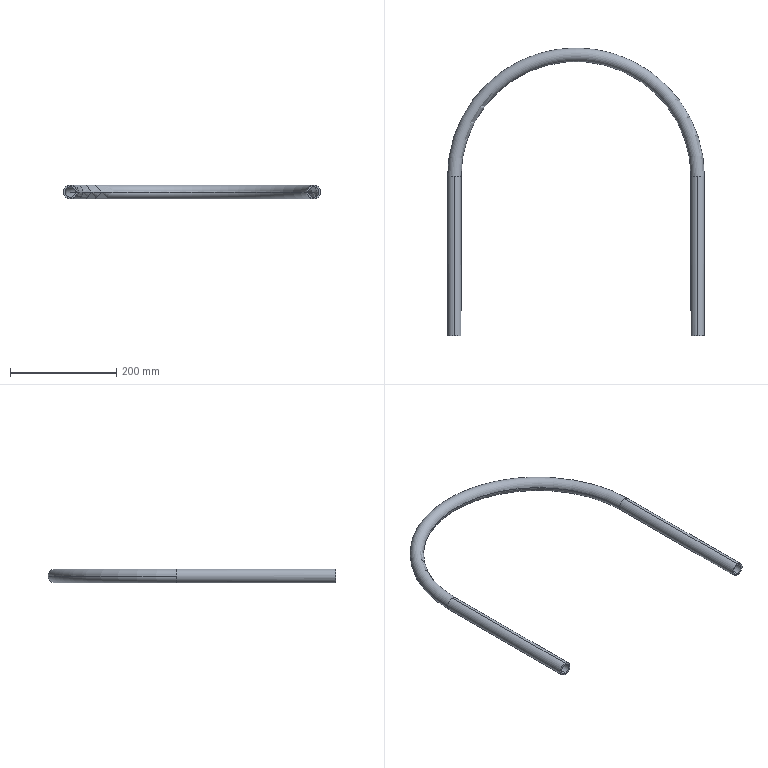Part | STEP file | 51E-01211JG10 | 1 solid | 14 faces | box 483.4 x 541.7 x 25.4 mm | volume 262302 mm3 | cylinder 8 | torus 4 | plane 2 | commonest cylinder face diameters 19.8 x4 25.4 x4
STEP:
#1=CARTESIAN_POINT('',(-238.9,300.,0.));
#2=VERTEX_POINT('',#1);
#3=CARTESIAN_POINT('',(-229.,300.,9.9));
#4=VERTEX_POINT('',#3);
#5=CARTESIAN_POINT('',(-229.,300.,0.));
#6=DIRECTION('',(0.,-1.,0.));
#7=AXIS2_PLACEMENT_3D('',#5,#6,$);
#8=CIRCLE('',#7,9.9);
#9=EDGE_CURVE('',#2,#4,#8,.F.);
#10=ORIENTED_EDGE('',*,*,#9,.F.);
#11=CARTESIAN_POINT('',(238.9,300.,0.));
#12=VERTEX_POINT('',#11);
#13=CARTESIAN_POINT('',(0.,300.,0.));
#14=DIRECTION('',(0.,0.,-1.));
#15=AXIS2_PLACEMENT_3D('',#13,#14,$);
#16=CIRCLE('',#15,238.9);
#17=EDGE_CURVE('',#2,#12,#16,.T.);
#18=ORIENTED_EDGE('',*,*,#17,.T.);
#19=CARTESIAN_POINT('',(229.,300.,9.9));
#20=VERTEX_POINT('',#19);
#21=CARTESIAN_POINT('',(229.,300.,0.));
#22=DIRECTION('',(0.,1.,0.));
#23=AXIS2_PLACEMENT_3D('',#21,#22,$);
#24=CIRCLE('',#23,9.9);
#25=EDGE_CURVE('',#12,#20,#24,.F.);
#26=ORIENTED_EDGE('',*,*,#25,.T.);
#27=CARTESIAN_POINT('',(219.1,300.,0.));
#28=VERTEX_POINT('',#27);
#29=CARTESIAN_POINT('',(229.,300.,0.));
#30=DIRECTION('',(0.,1.,0.));
#31=AXIS2_PLACEMENT_3D('',#29,#30,$);
#32=CIRCLE('',#31,9.9);
#33=EDGE_CURVE('',#20,#28,#32,.F.);
#34=ORIENTED_EDGE('',*,*,#33,.T.);
#35=CARTESIAN_POINT('',(-219.1,300.,0.));
#36=VERTEX_POINT('',#35);
#37=CARTESIAN_POINT('',(0.,300.,0.));
#38=DIRECTION('',(0.,0.,-1.));
#39=AXIS2_PLACEMENT_3D('',#37,#38,$);
#40=CIRCLE('',#39,219.1);
#41=EDGE_CURVE('',#36,#28,#40,.T.);
#42=ORIENTED_EDGE('',*,*,#41,.F.);
#43=CARTESIAN_POINT('',(-229.,300.,0.));
#44=DIRECTION('',(0.,-1.,0.));
#45=AXIS2_PLACEMENT_3D('',#43,#44,$);
#46=CIRCLE('',#45,9.9);
#47=EDGE_CURVE('',#4,#36,#46,.F.);
#48=ORIENTED_EDGE('',*,*,#47,.F.);
#49=EDGE_LOOP('',(#10,#18,#26,#34,#42,#48));
#50=FACE_OUTER_BOUND('',#49,.T.);
#51=CARTESIAN_POINT('',(0.,300.,0.));
#52=DIRECTION('',(0.,0.,-1.));
#53=DIRECTION('',(-1.,0.,0.));
#54=AXIS2_PLACEMENT_3D('',#51,#52,#53);
#55=TOROIDAL_SURFACE('',#54,229.,9.9);
#56=ADVANCED_FACE('',(#50),#55,.F.);
#57=CARTESIAN_POINT('',(-229.,300.,-9.9));
#58=VERTEX_POINT('',#57);
#59=CARTESIAN_POINT('',(-229.,300.,0.));
#60=DIRECTION('',(0.,-1.,0.));
#61=AXIS2_PLACEMENT_3D('',#59,#60,$);
#62=CIRCLE('',#61,9.9);
#63=EDGE_CURVE('',#58,#2,#62,.F.);
#64=ORIENTED_EDGE('',*,*,#63,.T.);
#65=ORIENTED_EDGE('',*,*,#9,.T.);
#66=CARTESIAN_POINT('',(-229.,0.,9.9));
#67=VERTEX_POINT('',#66);
#68=CARTESIAN_POINT('',(-229.,300.,9.9));
#69=DIRECTION('',(0.,-1.,0.));
#70=VECTOR('',#69,1.);
#71=LINE('',#68,#70);
#72=EDGE_CURVE('',#4,#67,#71,.T.);
#73=ORIENTED_EDGE('',*,*,#72,.T.);
#74=CARTESIAN_POINT('',(-229.,0.,-9.9));
#75=VERTEX_POINT('',#74);
#76=CARTESIAN_POINT('',(-229.,0.,0.));
#77=DIRECTION('',(0.,-1.,0.));
#78=AXIS2_PLACEMENT_3D('',#76,#77,$);
#79=CIRCLE('',#78,9.9);
#80=EDGE_CURVE('',#75,#67,#79,.F.);
#81=ORIENTED_EDGE('',*,*,#80,.F.);
#82=CARTESIAN_POINT('',(-229.,300.,-9.9));
#83=DIRECTION('',(0.,-1.,0.));
#84=VECTOR('',#83,1.);
#85=LINE('',#82,#84);
#86=EDGE_CURVE('',#58,#75,#85,.T.);
#87=ORIENTED_EDGE('',*,*,#86,.F.);
#88=EDGE_LOOP('',(#64,#65,#73,#81,#87));
#89=FACE_OUTER_BOUND('',#88,.T.);
#90=CARTESIAN_POINT('',(-229.,300.,0.));
#91=DIRECTION('',(0.,-1.,0.));
#92=DIRECTION('',(0.,0.,1.));
#93=AXIS2_PLACEMENT_3D('',#90,#91,#92);
#94=CYLINDRICAL_SURFACE('',#93,9.9);
#95=ADVANCED_FACE('',(#89),#94,.F.);
#96=ORIENTED_EDGE('',*,*,#17,.F.);
#97=ORIENTED_EDGE('',*,*,#63,.F.);
#98=CARTESIAN_POINT('',(-229.,300.,0.));
#99=DIRECTION('',(0.,-1.,0.));
#100=AXIS2_PLACEMENT_3D('',#98,#99,$);
#101=CIRCLE('',#100,9.9);
#102=EDGE_CURVE('',#36,#58,#101,.F.);
#103=ORIENTED_EDGE('',*,*,#102,.F.);
#104=ORIENTED_EDGE('',*,*,#41,.T.);
#105=CARTESIAN_POINT('',(229.,300.,-9.9));
#106=VERTEX_POINT('',#105);
#107=CARTESIAN_POINT('',(229.,300.,0.));
#108=DIRECTION('',(0.,1.,0.));
#109=AXIS2_PLACEMENT_3D('',#107,#108,$);
#110=CIRCLE('',#109,9.9);
#111=EDGE_CURVE('',#28,#106,#110,.F.);
#112=ORIENTED_EDGE('',*,*,#111,.T.);
#113=CARTESIAN_POINT('',(229.,300.,0.));
#114=DIRECTION('',(0.,1.,0.));
#115=AXIS2_PLACEMENT_3D('',#113,#114,$);
#116=CIRCLE('',#115,9.9);
#117=EDGE_CURVE('',#106,#12,#116,.F.);
#118=ORIENTED_EDGE('',*,*,#117,.T.);
#119=EDGE_LOOP('',(#96,#97,#103,#104,#112,#118));
#120=FACE_OUTER_BOUND('',#119,.T.);
#121=CARTESIAN_POINT('',(0.,300.,0.));
#122=DIRECTION('',(0.,0.,-1.));
#123=DIRECTION('',(-1.,0.,0.));
#124=AXIS2_PLACEMENT_3D('',#121,#122,#123);
#125=TOROIDAL_SURFACE('',#124,229.,9.9);
#126=ADVANCED_FACE('',(#120),#125,.F.);
#127=CARTESIAN_POINT('',(229.,0.,9.9));
#128=VERTEX_POINT('',#127);
#129=CARTESIAN_POINT('',(229.,300.,9.9));
#130=DIRECTION('',(0.,-1.,0.));
#131=VECTOR('',#130,1.);
#132=LINE('',#129,#131);
#133=EDGE_CURVE('',#20,#128,#132,.T.);
#134=ORIENTED_EDGE('',*,*,#133,.F.);
#135=ORIENTED_EDGE('',*,*,#25,.F.);
#136=ORIENTED_EDGE('',*,*,#117,.F.);
#137=CARTESIAN_POINT('',(229.,0.,-9.9));
#138=VERTEX_POINT('',#137);
#139=CARTESIAN_POINT('',(229.,300.,-9.9));
#140=DIRECTION('',(0.,-1.,0.));
#141=VECTOR('',#140,1.);
#142=LINE('',#139,#141);
#143=EDGE_CURVE('',#106,#138,#142,.T.);
#144=ORIENTED_EDGE('',*,*,#143,.T.);
#145=CARTESIAN_POINT('',(229.,0.,0.));
#146=DIRECTION('',(0.,-1.,0.));
#147=AXIS2_PLACEMENT_3D('',#145,#146,$);
#148=CIRCLE('',#147,9.9);
#149=EDGE_CURVE('',#138,#128,#148,.T.);
#150=ORIENTED_EDGE('',*,*,#149,.T.);
#151=EDGE_LOOP('',(#134,#135,#136,#144,#150));
#152=FACE_OUTER_BOUND('',#151,.T.);
#153=CARTESIAN_POINT('',(229.,300.,0.));
#154=DIRECTION('',(0.,-1.,0.));
#155=DIRECTION('',(0.,0.,-1.));
#156=AXIS2_PLACEMENT_3D('',#153,#154,#155);
#157=CYLINDRICAL_SURFACE('',#156,9.9);
#158=ADVANCED_FACE('',(#152),#157,.F.);
#159=ORIENTED_EDGE('',*,*,#33,.F.);
#160=ORIENTED_EDGE('',*,*,#133,.T.);
#161=CARTESIAN_POINT('',(229.,0.,0.));
#162=DIRECTION('',(0.,-1.,0.));
#163=AXIS2_PLACEMENT_3D('',#161,#162,$);
#164=CIRCLE('',#163,9.9);
#165=EDGE_CURVE('',#128,#138,#164,.T.);
#166=ORIENTED_EDGE('',*,*,#165,.T.);
#167=ORIENTED_EDGE('',*,*,#143,.F.);
#168=ORIENTED_EDGE('',*,*,#111,.F.);
#169=EDGE_LOOP('',(#159,#160,#166,#167,#168));
#170=FACE_OUTER_BOUND('',#169,.T.);
#171=CARTESIAN_POINT('',(229.,300.,0.));
#172=DIRECTION('',(0.,-1.,0.));
#173=DIRECTION('',(0.,0.,1.));
#174=AXIS2_PLACEMENT_3D('',#171,#172,#173);
#175=CYLINDRICAL_SURFACE('',#174,9.9);
#176=ADVANCED_FACE('',(#170),#175,.F.);
#177=ORIENTED_EDGE('',*,*,#72,.F.);
#178=ORIENTED_EDGE('',*,*,#47,.T.);
#179=ORIENTED_EDGE('',*,*,#102,.T.);
#180=ORIENTED_EDGE('',*,*,#86,.T.);
#181=CARTESIAN_POINT('',(-229.,0.,0.));
#182=DIRECTION('',(0.,-1.,0.));
#183=AXIS2_PLACEMENT_3D('',#181,#182,$);
#184=CIRCLE('',#183,9.9);
#185=EDGE_CURVE('',#67,#75,#184,.F.);
#186=ORIENTED_EDGE('',*,*,#185,.F.);
#187=EDGE_LOOP('',(#177,#178,#179,#180,#186));
#188=FACE_OUTER_BOUND('',#187,.T.);
#189=CARTESIAN_POINT('',(-229.,300.,0.));
#190=DIRECTION('',(0.,-1.,0.));
#191=DIRECTION('',(0.,0.,-1.));
#192=AXIS2_PLACEMENT_3D('',#189,#190,#191);
#193=CYLINDRICAL_SURFACE('',#192,9.9);
#194=ADVANCED_FACE('',(#188),#193,.F.);
#195=CARTESIAN_POINT('',(-229.,0.,-12.7));
#196=VERTEX_POINT('',#195);
#197=CARTESIAN_POINT('',(-229.,0.,12.7));
#198=VERTEX_POINT('',#197);
#199=CARTESIAN_POINT('',(-229.,0.,0.));
#200=DIRECTION('',(0.,1.,0.));
#201=AXIS2_PLACEMENT_3D('',#199,#200,$);
#202=CIRCLE('',#201,12.7);
#203=EDGE_CURVE('',#196,#198,#202,.T.);
#204=ORIENTED_EDGE('',*,*,#203,.F.);
#205=CARTESIAN_POINT('',(-229.,0.,0.));
#206=DIRECTION('',(0.,1.,0.));
#207=AXIS2_PLACEMENT_3D('',#205,#206,$);
#208=CIRCLE('',#207,12.7);
#209=EDGE_CURVE('',#198,#196,#208,.T.);
#210=ORIENTED_EDGE('',*,*,#209,.F.);
#211=EDGE_LOOP('',(#204,#210));
#212=FACE_OUTER_BOUND('',#211,.T.);
#213=ORIENTED_EDGE('',*,*,#80,.T.);
#214=ORIENTED_EDGE('',*,*,#185,.T.);
#215=EDGE_LOOP('',(#213,#214));
#216=FACE_BOUND('',#215,.T.);
#217=CARTESIAN_POINT('',(-229.,0.,0.));
#218=DIRECTION('',(0.,1.,0.));
#219=DIRECTION('',(0.,0.,1.));
#220=AXIS2_PLACEMENT_3D('',#217,#218,#219);
#221=PLANE('',#220);
#222=ADVANCED_FACE('',(#212,#216),#221,.F.);
#223=CARTESIAN_POINT('',(229.,0.,-12.7));
#224=VERTEX_POINT('',#223);
#225=CARTESIAN_POINT('',(229.,0.,12.7));
#226=VERTEX_POINT('',#225);
#227=CARTESIAN_POINT('',(229.,0.,0.));
#228=DIRECTION('',(0.,-1.,0.));
#229=AXIS2_PLACEMENT_3D('',#227,#228,$);
#230=CIRCLE('',#229,12.7);
#231=EDGE_CURVE('',#224,#226,#230,.T.);
#232=ORIENTED_EDGE('',*,*,#231,.T.);
#233=CARTESIAN_POINT('',(229.,0.,0.));
#234=DIRECTION('',(0.,-1.,0.));
#235=AXIS2_PLACEMENT_3D('',#233,#234,$);
#236=CIRCLE('',#235,12.7);
#237=EDGE_CURVE('',#226,#224,#236,.T.);
#238=ORIENTED_EDGE('',*,*,#237,.T.);
#239=EDGE_LOOP('',(#232,#238));
#240=FACE_OUTER_BOUND('',#239,.T.);
#241=ORIENTED_EDGE('',*,*,#149,.F.);
#242=ORIENTED_EDGE('',*,*,#165,.F.);
#243=EDGE_LOOP('',(#241,#242));
#244=FACE_BOUND('',#243,.T.);
#245=CARTESIAN_POINT('',(229.,0.,0.));
#246=DIRECTION('',(0.,-1.,0.));
#247=DIRECTION('',(0.,0.,1.));
#248=AXIS2_PLACEMENT_3D('',#245,#246,#247);
#249=PLANE('',#248);
#250=ADVANCED_FACE('',(#240,#244),#249,.T.);
#251=CARTESIAN_POINT('',(-229.,300.,12.7));
#252=VERTEX_POINT('',#251);
#253=CARTESIAN_POINT('',(-229.,300.,12.7));
#254=DIRECTION('',(0.,-1.,0.));
#255=VECTOR('',#254,1.);
#256=LINE('',#253,#255);
#257=EDGE_CURVE('',#252,#198,#256,.T.);
#258=ORIENTED_EDGE('',*,*,#257,.F.);
#259=CARTESIAN_POINT('',(-241.7,300.,0.));
#260=VERTEX_POINT('',#259);
#261=CARTESIAN_POINT('',(-229.,300.,0.));
#262=DIRECTION('',(0.,-1.,0.));
#263=AXIS2_PLACEMENT_3D('',#261,#262,$);
#264=CIRCLE('',#263,12.7);
#265=EDGE_CURVE('',#260,#252,#264,.F.);
#266=ORIENTED_EDGE('',*,*,#265,.F.);
#267=CARTESIAN_POINT('',(-229.,300.,-12.7));
#268=VERTEX_POINT('',#267);
#269=CARTESIAN_POINT('',(-229.,300.,0.));
#270=DIRECTION('',(0.,-1.,0.));
#271=AXIS2_PLACEMENT_3D('',#269,#270,$);
#272=CIRCLE('',#271,12.7);
#273=EDGE_CURVE('',#268,#260,#272,.F.);
#274=ORIENTED_EDGE('',*,*,#273,.F.);
#275=CARTESIAN_POINT('',(-229.,300.,-12.7));
#276=DIRECTION('',(0.,-1.,0.));
#277=VECTOR('',#276,1.);
#278=LINE('',#275,#277);
#279=EDGE_CURVE('',#268,#196,#278,.T.);
#280=ORIENTED_EDGE('',*,*,#279,.T.);
#281=ORIENTED_EDGE('',*,*,#203,.T.);
#282=EDGE_LOOP('',(#258,#266,#274,#280,#281));
#283=FACE_OUTER_BOUND('',#282,.T.);
#284=CARTESIAN_POINT('',(-229.,300.,0.));
#285=DIRECTION('',(0.,-1.,0.));
#286=DIRECTION('',(0.,0.,1.));
#287=AXIS2_PLACEMENT_3D('',#284,#285,#286);
#288=CYLINDRICAL_SURFACE('',#287,12.7);
#289=ADVANCED_FACE('',(#283),#288,.T.);
#290=CARTESIAN_POINT('',(-216.3,300.,0.));
#291=VERTEX_POINT('',#290);
#292=CARTESIAN_POINT('',(-229.,300.,0.));
#293=DIRECTION('',(0.,-1.,0.));
#294=AXIS2_PLACEMENT_3D('',#292,#293,$);
#295=CIRCLE('',#294,12.7);
#296=EDGE_CURVE('',#252,#291,#295,.F.);
#297=ORIENTED_EDGE('',*,*,#296,.F.);
#298=ORIENTED_EDGE('',*,*,#257,.T.);
#299=ORIENTED_EDGE('',*,*,#209,.T.);
#300=ORIENTED_EDGE('',*,*,#279,.F.);
#301=CARTESIAN_POINT('',(-229.,300.,0.));
#302=DIRECTION('',(0.,-1.,0.));
#303=AXIS2_PLACEMENT_3D('',#301,#302,$);
#304=CIRCLE('',#303,12.7);
#305=EDGE_CURVE('',#291,#268,#304,.F.);
#306=ORIENTED_EDGE('',*,*,#305,.F.);
#307=EDGE_LOOP('',(#297,#298,#299,#300,#306));
#308=FACE_OUTER_BOUND('',#307,.T.);
#309=CARTESIAN_POINT('',(-229.,300.,0.));
#310=DIRECTION('',(0.,-1.,0.));
#311=DIRECTION('',(0.,0.,-1.));
#312=AXIS2_PLACEMENT_3D('',#309,#310,#311);
#313=CYLINDRICAL_SURFACE('',#312,12.7);
#314=ADVANCED_FACE('',(#308),#313,.T.);
#315=CARTESIAN_POINT('',(229.,300.,-12.7));
#316=VERTEX_POINT('',#315);
#317=CARTESIAN_POINT('',(241.7,300.,0.));
#318=VERTEX_POINT('',#317);
#319=CARTESIAN_POINT('',(229.,300.,0.));
#320=DIRECTION('',(0.,-1.,0.));
#321=AXIS2_PLACEMENT_3D('',#319,#320,$);
#322=CIRCLE('',#321,12.7);
#323=EDGE_CURVE('',#316,#318,#322,.T.);
#324=ORIENTED_EDGE('',*,*,#323,.T.);
#325=CARTESIAN_POINT('',(229.,300.,12.7));
#326=VERTEX_POINT('',#325);
#327=CARTESIAN_POINT('',(229.,300.,0.));
#328=DIRECTION('',(0.,-1.,0.));
#329=AXIS2_PLACEMENT_3D('',#327,#328,$);
#330=CIRCLE('',#329,12.7);
#331=EDGE_CURVE('',#318,#326,#330,.T.);
#332=ORIENTED_EDGE('',*,*,#331,.T.);
#333=CARTESIAN_POINT('',(229.,300.,12.7));
#334=DIRECTION('',(0.,-1.,0.));
#335=VECTOR('',#334,1.);
#336=LINE('',#333,#335);
#337=EDGE_CURVE('',#326,#226,#336,.T.);
#338=ORIENTED_EDGE('',*,*,#337,.T.);
#339=ORIENTED_EDGE('',*,*,#231,.F.);
#340=CARTESIAN_POINT('',(229.,300.,-12.7));
#341=DIRECTION('',(0.,-1.,0.));
#342=VECTOR('',#341,1.);
#343=LINE('',#340,#342);
#344=EDGE_CURVE('',#316,#224,#343,.T.);
#345=ORIENTED_EDGE('',*,*,#344,.F.);
#346=EDGE_LOOP('',(#324,#332,#338,#339,#345));
#347=FACE_OUTER_BOUND('',#346,.T.);
#348=CARTESIAN_POINT('',(229.,300.,0.));
#349=DIRECTION('',(0.,-1.,0.));
#350=DIRECTION('',(0.,0.,-1.));
#351=AXIS2_PLACEMENT_3D('',#348,#349,#350);
#352=CYLINDRICAL_SURFACE('',#351,12.7);
#353=ADVANCED_FACE('',(#347),#352,.T.);
#354=ORIENTED_EDGE('',*,*,#337,.F.);
#355=CARTESIAN_POINT('',(216.3,300.,0.));
#356=VERTEX_POINT('',#355);
#357=CARTESIAN_POINT('',(229.,300.,0.));
#358=DIRECTION('',(0.,-1.,0.));
#359=AXIS2_PLACEMENT_3D('',#357,#358,$);
#360=CIRCLE('',#359,12.7);
#361=EDGE_CURVE('',#326,#356,#360,.T.);
#362=ORIENTED_EDGE('',*,*,#361,.T.);
#363=CARTESIAN_POINT('',(229.,300.,0.));
#364=DIRECTION('',(0.,-1.,0.));
#365=AXIS2_PLACEMENT_3D('',#363,#364,$);
#366=CIRCLE('',#365,12.7);
#367=EDGE_CURVE('',#356,#316,#366,.T.);
#368=ORIENTED_EDGE('',*,*,#367,.T.);
#369=ORIENTED_EDGE('',*,*,#344,.T.);
#370=ORIENTED_EDGE('',*,*,#237,.F.);
#371=EDGE_LOOP('',(#354,#362,#368,#369,#370));
#372=FACE_OUTER_BOUND('',#371,.T.);
#373=CARTESIAN_POINT('',(229.,300.,0.));
#374=DIRECTION('',(0.,-1.,0.));
#375=DIRECTION('',(0.,0.,1.));
#376=AXIS2_PLACEMENT_3D('',#373,#374,#375);
#377=CYLINDRICAL_SURFACE('',#376,12.7);
#378=ADVANCED_FACE('',(#372),#377,.T.);
#379=CARTESIAN_POINT('',(0.,300.,0.));
#380=DIRECTION('',(0.,0.,-1.));
#381=AXIS2_PLACEMENT_3D('',#379,#380,$);
#382=CIRCLE('',#381,241.7);
#383=EDGE_CURVE('',#260,#318,#382,.T.);
#384=ORIENTED_EDGE('',*,*,#383,.F.);
#385=ORIENTED_EDGE('',*,*,#265,.T.);
#386=ORIENTED_EDGE('',*,*,#296,.T.);
#387=CARTESIAN_POINT('',(0.,300.,0.));
#388=DIRECTION('',(0.,0.,-1.));
#389=AXIS2_PLACEMENT_3D('',#387,#388,$);
#390=CIRCLE('',#389,216.3);
#391=EDGE_CURVE('',#291,#356,#390,.T.);
#392=ORIENTED_EDGE('',*,*,#391,.T.);
#393=ORIENTED_EDGE('',*,*,#361,.F.);
#394=ORIENTED_EDGE('',*,*,#331,.F.);
#395=EDGE_LOOP('',(#384,#385,#386,#392,#393,#394));
#396=FACE_OUTER_BOUND('',#395,.T.);
#397=CARTESIAN_POINT('',(0.,300.,0.));
#398=DIRECTION('',(0.,0.,-1.));
#399=DIRECTION('',(-1.,0.,0.));
#400=AXIS2_PLACEMENT_3D('',#397,#398,#399);
#401=TOROIDAL_SURFACE('',#400,229.,12.7);
#402=ADVANCED_FACE('',(#396),#401,.T.);
#403=ORIENTED_EDGE('',*,*,#273,.T.);
#404=ORIENTED_EDGE('',*,*,#383,.T.);
#405=ORIENTED_EDGE('',*,*,#323,.F.);
#406=ORIENTED_EDGE('',*,*,#367,.F.);
#407=ORIENTED_EDGE('',*,*,#391,.F.);
#408=ORIENTED_EDGE('',*,*,#305,.T.);
#409=EDGE_LOOP('',(#403,#404,#405,#406,#407,#408));
#410=FACE_OUTER_BOUND('',#409,.T.);
#411=CARTESIAN_POINT('',(0.,300.,0.));
#412=DIRECTION('',(0.,0.,-1.));
#413=DIRECTION('',(-1.,0.,0.));
#414=AXIS2_PLACEMENT_3D('',#411,#412,#413);
#415=TOROIDAL_SURFACE('',#414,229.,12.7);
#416=ADVANCED_FACE('',(#410),#415,.T.);
#417=CLOSED_SHELL('',(#56,#95,#126,#158,#176,#194,#222,#250,#289,#314,#353,#378,#402,#416));
#418=MANIFOLD_SOLID_BREP('',#417);
#419=(LENGTH_UNIT()NAMED_UNIT(*)SI_UNIT(.MILLI.,.METRE.));
#420=UNCERTAINTY_MEASURE_WITH_UNIT(LENGTH_MEASURE(0.005),#419,'','');
#421=(NAMED_UNIT(*)PLANE_ANGLE_UNIT()SI_UNIT($,.RADIAN.));
#422=(NAMED_UNIT(*)SI_UNIT($,.STERADIAN.)SOLID_ANGLE_UNIT());
#423=(GEOMETRIC_REPRESENTATION_CONTEXT(3)GLOBAL_UNCERTAINTY_ASSIGNED_CONTEXT((#420))GLOBAL_UNIT_ASSIGNED_CONTEXT((#419,#421,#422))REPRESENTATION_CONTEXT('',''));
#424=ADVANCED_BREP_SHAPE_REPRESENTATION('',(#418),#423);